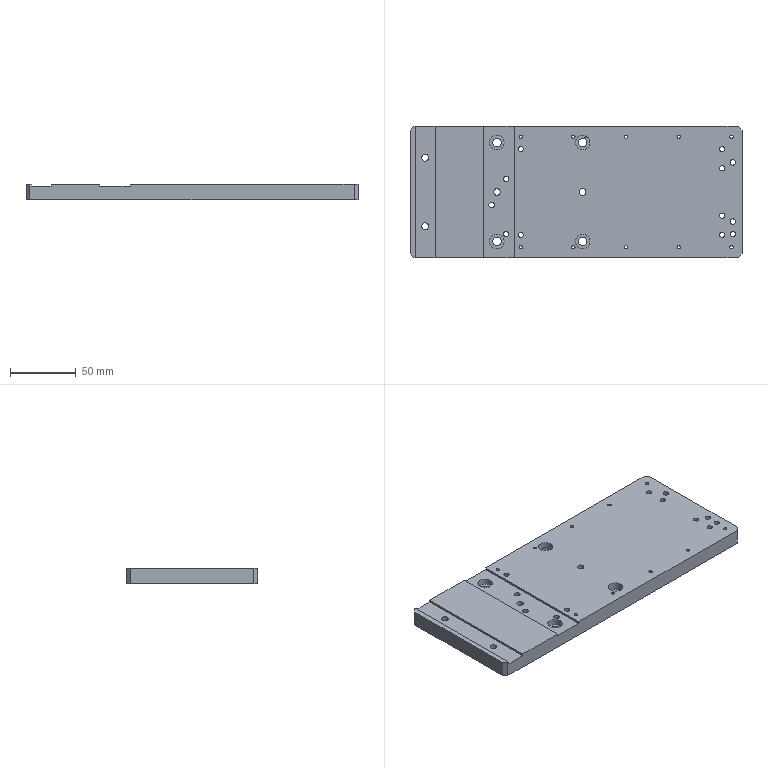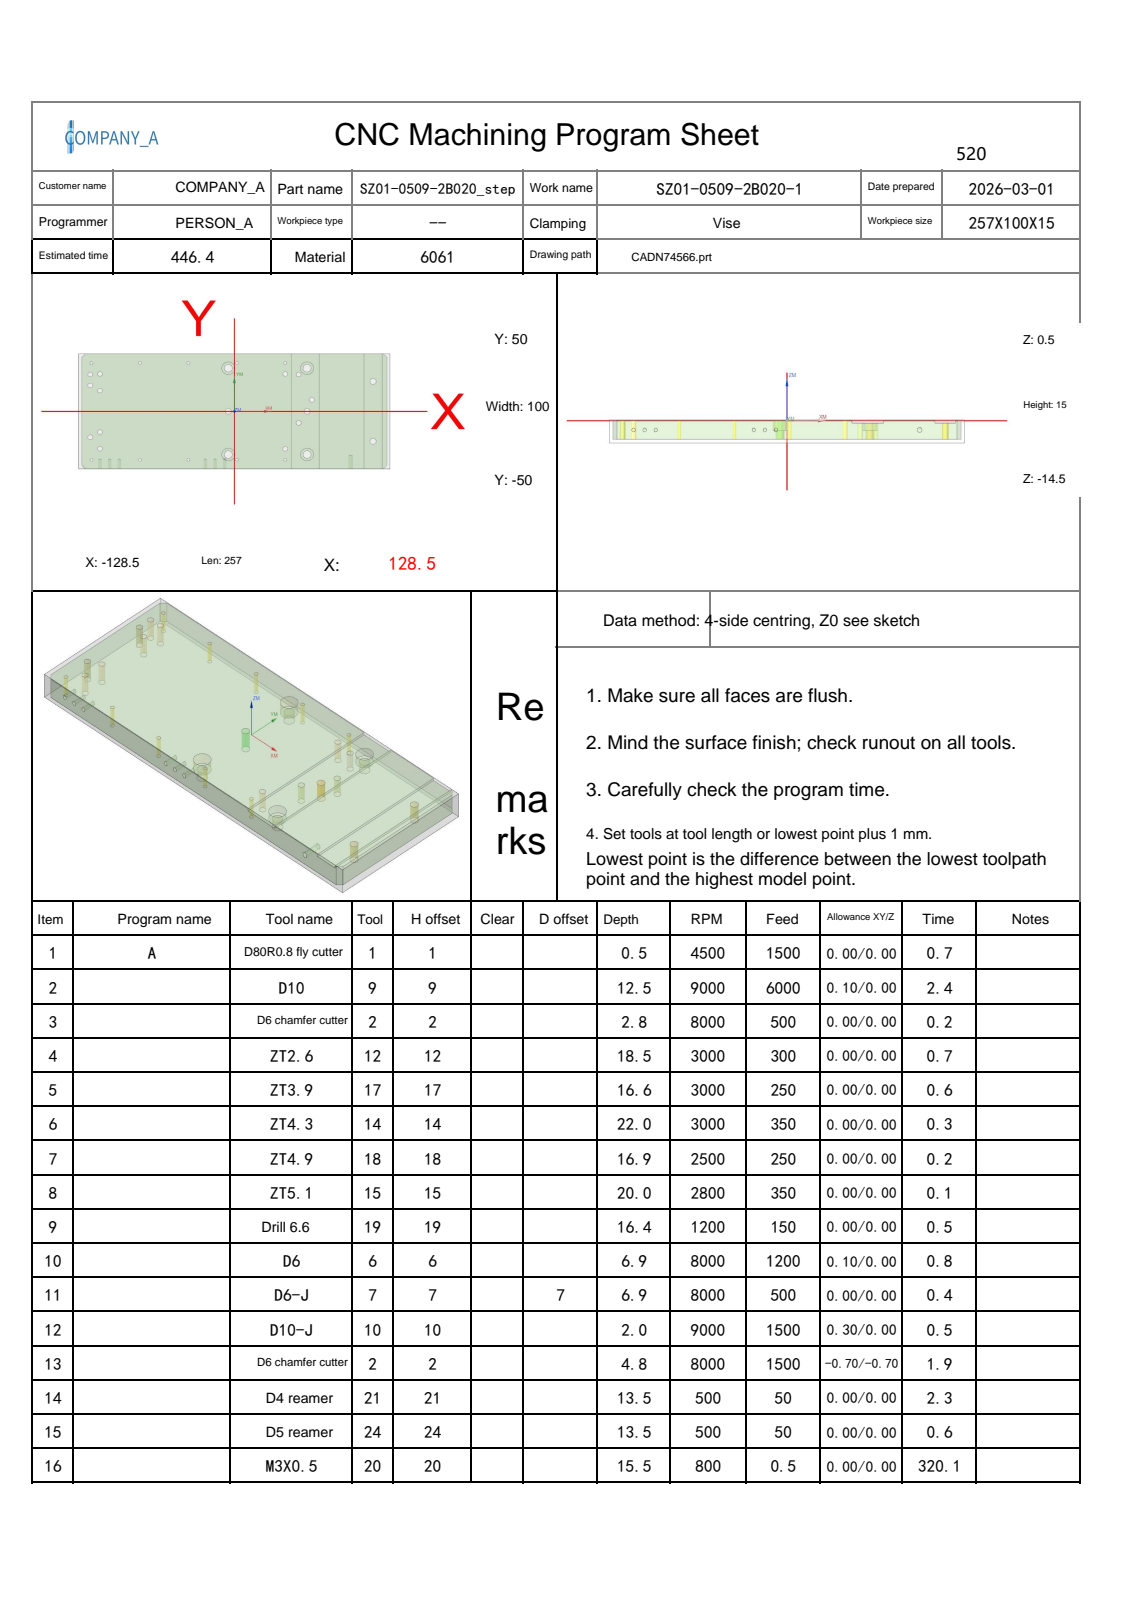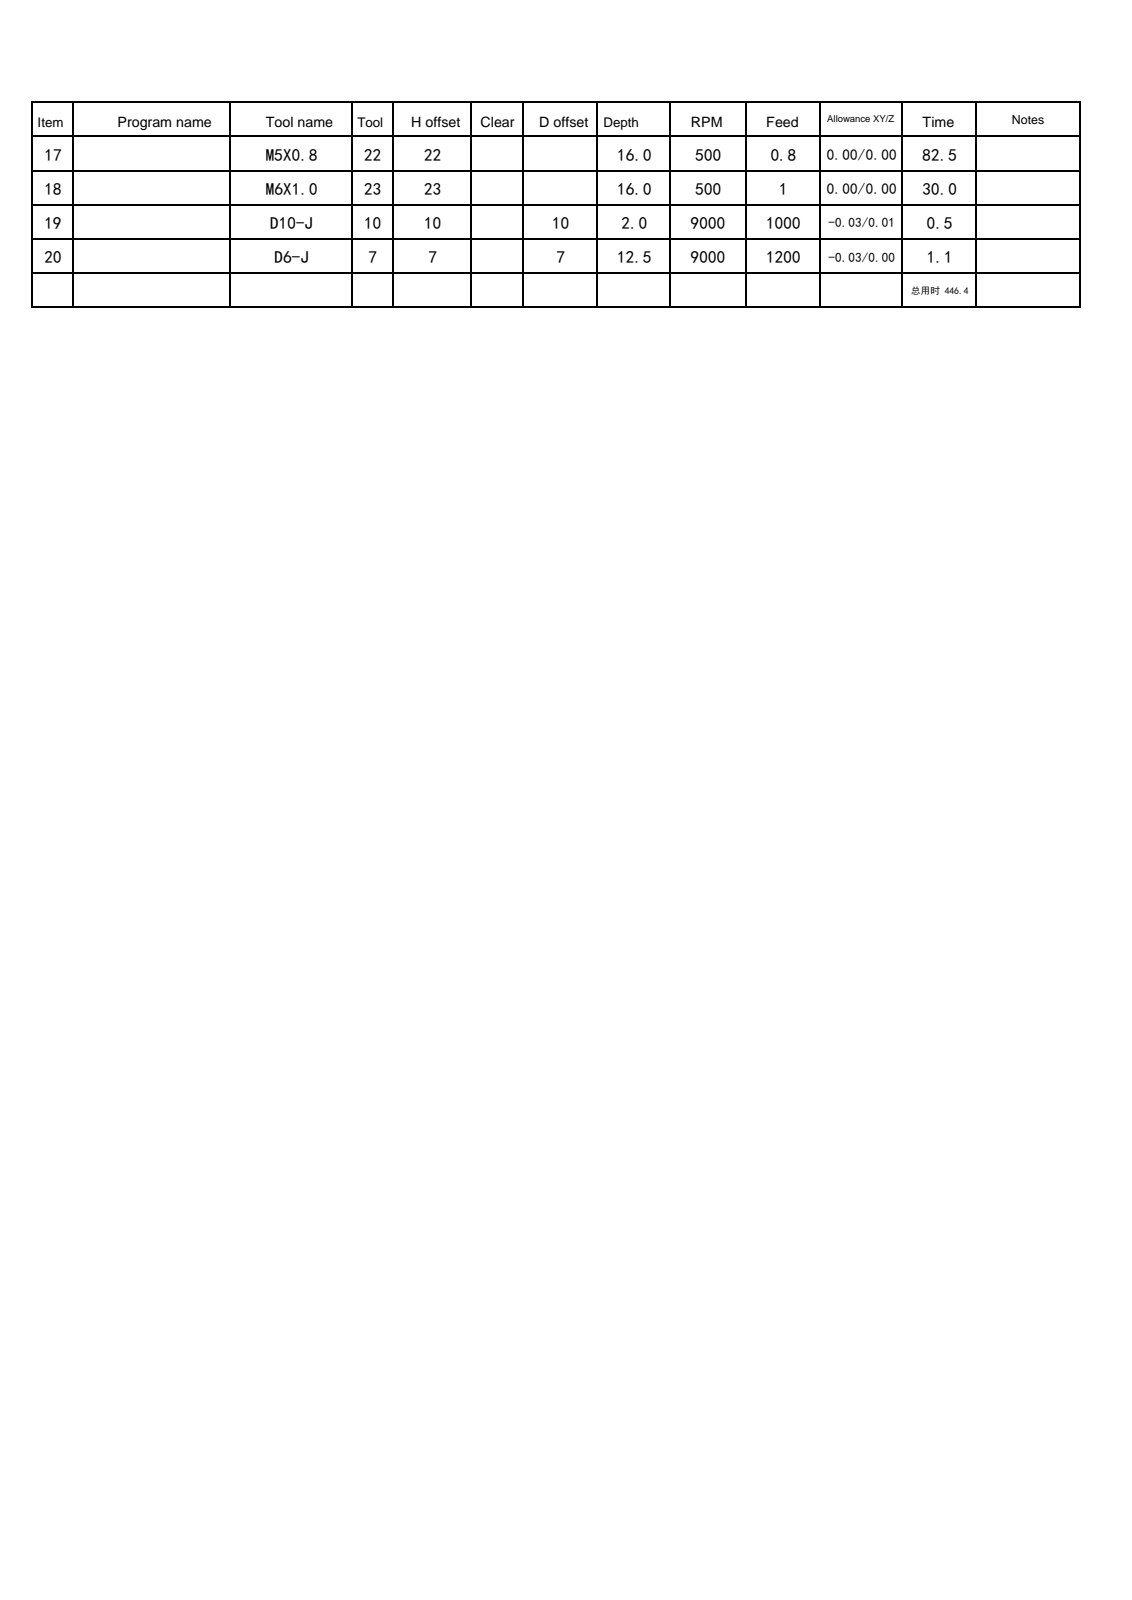NC program | NX | posted by the shop | part box 252 x 100 x 12 mm
Whole program:
%
O0001
(Machine time: 855.61 MIN)
(===Total Tool:17===)
(T1=D80R0.8 fly cutter D=80.  R=0.8  D-  H01 Z=-0.   )
(T9=D10     D=10.  R=0.   D-  H09 Z=-12.  )
(T2=D6 chamfer cutter   D=6.   R=0.   D-  H02 Z=-4.3  )
(T12=ZT2.6  D=2.6  DR_a=118 D-  H12 Z=-18.  )
(T17=ZT3.9  D=3.9  DR_a=120 D-  H17 Z=-16.13)
(T14=ZT4.3  D=4.3  DR_a=118 D-  H14 Z=-21.5 )
(T18=ZT4.9  D=4.9  DR_a=120 D-  H18 Z=-16.41)
(T15=ZT5.1  D=5.1  DR_a=118 D-  H15 Z=-19.53)
(T19=drill 6.6  D=6.6  DR_a=120 D-  H19 Z=-15.91)
(T6=D6      D=6.   R=0.   D-  H06 Z=-6.4  )
(T7=D6-J    D=6.   R=0.   D7  H07 Z=-12.  )
(T10=D10-J  D=10.  R=0.   D-  H10 Z=-1.5  )
(T21=D4 reamer   D=4.   DR_a=180 D-  H21 Z=-13.  )
(T24=D5 reamer   D=5.   DR_a=180 D-  H24 Z=-13.  )
(T20=M3X0.5 D=2.5  DR_a=180 D-  H20 Z=-15.  )
(T22=M5X0.8 D=4.2  DR_a=180 D-  H22 Z=-15.5 )
(T23=M6X1.0 D=5.   DR_a=180 D-  H23 Z=-15.5 )
G80 G90 G17 G49 G40
G91 G28 Z0
M01
N1 T01 M06
(D80R0.8 fly cutter  D=80. R=0.8 H=01 ce=0.00 di=0.00)
G00 G90 G54 X171. Y-45. M03 S4500
G43 H01 Z50.
M08
Z2.
G01 Z0.0 F1500.
X166.
X-166.
Y0.0
X166.
Y45.
X-166.
X-171.
Z2.
G00 Z50.
G91 G28 Z0.0
M05
M09
G91 G28 Z0.0
M01
N2 T09 M06
(D10  D=10. R=0. H=09 ce=0.10 di=0.00)
G00 G90 G54 X0.0 Y-55.1 M03 S8000
G43 H09 Z50.
M08
Z.5
G01 X-123. Z.368 F6000.
G02 X-126.606 Y-53.606 Z.364 I0.0 J5.1
G01 X-129.606 Y-50.606 Z.359
G02 X-131.1 Y-47. Z.355 I3.606 J3.606
G01 Y47. Z.254
G02 X-129.606 Y50.606 Z.25 I5.1 J0.0
G01 X-126.606 Y53.606 Z.245
G02 X-123. Y55.1 Z.241 I3.606 J-3.606
G01 X123. Z-.022
G02 X126.606 Y53.606 Z-.027 I0.0 J-5.1
G01 X129.606 Y50.606 Z-.031
G02 X131.1 Y47. Z-.036 I-3.606 J-3.606
G01 Y-47. Z-.136
G02 X129.606 Y-50.606 Z-.141 I-5.1 J0.0
G01 X126.606 Y-53.606 Z-.145
G02 X123. Y-55.1 Z-.149 I-3.606 J3.606
G01 X-123. Z-.413
G02 X-126.606 Y-53.606 Z-.417 I0.0 J5.1
G01 X-129.606 Y-50.606 Z-.422
G02 X-131.1 Y-47. Z-.426 I3.606 J3.606
G01 Y47. Z-.527
G02 X-129.606 Y50.606 Z-.531 I5.1 J0.0
G01 X-126.606 Y53.606 Z-.536
G02 X-123. Y55.1 Z-.54 I3.606 J-3.606
G01 X123. Z-.804
G02 X126.606 Y53.606 Z-.808 I0.0 J-5.1
G01 X129.606 Y50.606 Z-.813
G02 X131.1 Y47. Z-.817 I-3.606 J-3.606
G01 Y-47. Z-.918
G02 X129.606 Y-50.606 Z-.922 I-5.1 J0.0
G01 X126.606 Y-53.606 Z-.926
G02 X123. Y-55.1 Z-.931 I-3.606 J3.606
G01 X-123. Z-1.194
G02 X-126.606 Y-53.606 Z-1.199 I0.0 J5.1
G01 X-129.606 Y-50.606 Z-1.203
G02 X-131.1 Y-47. Z-1.207 I3.606 J3.606
G01 Y47. Z-1.308
G02 X-129.606 Y50.606 Z-1.312 I5.1 J0.0
G01 X-126.606 Y53.606 Z-1.317
G02 X-123. Y55.1 Z-1.321 I3.606 J-3.606
G01 X123. Z-1.585
G02 X126.606 Y53.606 Z-1.589 I0.0 J-5.1
G01 X129.606 Y50.606 Z-1.594
G02 X131.1 Y47. Z-1.598 I-3.606 J-3.606
G01 Y-47. Z-1.699
G02 X129.606 Y-50.606 Z-1.703 I-5.1 J0.0
G01 X126.606 Y-53.606 Z-1.708
G02 X123. Y-55.1 Z-1.712 I-3.606 J3.606
G01 X-123. Z-1.976
G02 X-126.606 Y-53.606 Z-1.98 I0.0 J5.1
G01 X-129.606 Y-50.606 Z-1.984
G02 X-131.1 Y-47. Z-1.989 I3.606 J3.606
G01 Y47. Z-2.089
G02 X-129.606 Y50.606 Z-2.094 I5.1 J0.0
G01 X-126.606 Y53.606 Z-2.098
G02 X-123. Y55.1 Z-2.103 I3.606 J-3.606
G01 X123. Z-2.366
G02 X126.606 Y53.606 Z-2.37 I0.0 J-5.1
G01 X129.606 Y50.606 Z-2.375
G02 X131.1 Y47. Z-2.379 I-3.606 J-3.606
G01 Y-47. Z-2.48
G02 X129.606 Y-50.606 Z-2.484 I-5.1 J0.0
G01 X126.606 Y-53.606 Z-2.489
G02 X123. Y-55.1 Z-2.493 I-3.606 J3.606
G01 X-123. Z-2.757
G02 X-126.606 Y-53.606 Z-2.761 I0.0 J5.1
G01 X-129.606 Y-50.606 Z-2.766
G02 X-131.1 Y-47. Z-2.77 I3.606 J3.606
G01 Y47. Z-2.871
G02 X-129.606 Y50.606 Z-2.875 I5.1 J0.0
G01 X-126.606 Y53.606 Z-2.88
G02 X-123. Y55.1 Z-2.884 I3.606 J-3.606
G01 X123. Z-3.147
G02 X126.606 Y53.606 Z-3.152 I0.0 J-5.1
G01 X129.606 Y50.606 Z-3.156
G02 X131.1 Y47. Z-3.161 I-3.606 J-3.606
G01 Y-47. Z-3.261
G02 X129.606 Y-50.606 Z-3.266 I-5.1 J0.0
G01 X126.606 Y-53.606 Z-3.27
G02 X123. Y-55.1 Z-3.274 I-3.606 J3.606
G01 X-123. Z-3.538
G02 X-126.606 Y-53.606 Z-3.542 I0.0 J5.1
G01 X-129.606 Y-50.606 Z-3.547
G02 X-131.1 Y-47. Z-3.551 I3.606 J3.606
G01 Y47. Z-3.652
G02 X-129.606 Y50.606 Z-3.656 I5.1 J0.0
G01 X-126.606 Y53.606 Z-3.661
G02 X-123. Y55.1 Z-3.665 I3.606 J-3.606
G01 X123. Z-3.929
G02 X126.606 Y53.606 Z-3.933 I0.0 J-5.1
G01 X129.606 Y50.606 Z-3.938
G02 X131.1 Y47. Z-3.942 I-3.606 J-3.606
G01 Y-47. Z-4.043
G02 X129.606 Y-50.606 Z-4.047 I-5.1 J0.0
G01 X126.606 Y-53.606 Z-4.051
G02 X123. Y-55.1 Z-4.056 I-3.606 J3.606
G01 X-123. Z-4.319
G02 X-126.606 Y-53.606 Z-4.324 I0.0 J5.1
G01 X-129.606 Y-50.606 Z-4.328
G02 X-131.1 Y-47. Z-4.332 I3.606 J3.606
G01 Y47. Z-4.433
G02 X-129.606 Y50.606 Z-4.437 I5.1 J0.0
G01 X-126.606 Y53.606 Z-4.442
G02 X-123. Y55.1 Z-4.446 I3.606 J-3.606
G01 X123. Z-4.71
G02 X126.606 Y53.606 Z-4.714 I0.0 J-5.1
G01 X129.606 Y50.606 Z-4.719
G02 X131.1 Y47. Z-4.723 I-3.606 J-3.606
G01 Y-47. Z-4.824
G02 X129.606 Y-50.606 Z-4.828 I-5.1 J0.0
G01 X126.606 Y-53.606 Z-4.833
G02 X123. Y-55.1 Z-4.837 I-3.606 J3.606
G01 X-123. Z-5.101
G02 X-126.606 Y-53.606 Z-5.105 I0.0 J5.1
G01 X-129.606 Y-50.606 Z-5.109
G02 X-131.1 Y-47. Z-5.114 I3.606 J3.606
G01 Y47. Z-5.214
G02 X-129.606 Y50.606 Z-5.219 I5.1 J0.0
G01 X-126.606 Y53.606 Z-5.223
G02 X-123. Y55.1 Z-5.228 I3.606 J-3.606
G01 X123. Z-5.491
G02 X126.606 Y53.606 Z-5.495 I0.0 J-5.1
G01 X129.606 Y50.606 Z-5.5
G02 X131.1 Y47. Z-5.504 I-3.606 J-3.606
G01 Y-47. Z-5.605
G02 X129.606 Y-50.606 Z-5.609 I-5.1 J0.0
G01 X126.606 Y-53.606 Z-5.614
G02 X123. Y-55.1 Z-5.618 I-3.606 J3.606
G01 X-123. Z-5.882
G02 X-126.606 Y-53.606 Z-5.886 I0.0 J5.1
G01 X-129.606 Y-50.606 Z-5.891
G02 X-131.1 Y-47. Z-5.895 I3.606 J3.606
G01 Y47. Z-5.996
G02 X-129.606 Y50.606 Z-6. I5.1 J0.0
G01 X-126.606 Y53.606 Z-6.005
G02 X-123. Y55.1 Z-6.009 I3.606 J-3.606
G01 X123. Z-6.272
G02 X126.606 Y53.606 Z-6.277 I0.0 J-5.1
G01 X129.606 Y50.606 Z-6.281
G02 X131.1 Y47. Z-6.286 I-3.606 J-3.606
G01 Y-47. Z-6.386
G02 X129.606 Y-50.606 Z-6.391 I-5.1 J0.0
G01 X126.606 Y-53.606 Z-6.395
G02 X123. Y-55.1 Z-6.399 I-3.606 J3.606
G01 X-123. Z-6.663
G02 X-126.606 Y-53.606 Z-6.667 I0.0 J5.1
G01 X-129.606 Y-50.606 Z-6.672
G02 X-131.1 Y-47. Z-6.676 I3.606 J3.606
G01 Y47. Z-6.777
G02 X-129.606 Y50.606 Z-6.781 I5.1 J0.0
G01 X-126.606 Y53.606 Z-6.786
G02 X-123. Y55.1 Z-6.79 I3.606 J-3.606
G01 X123. Z-7.054
G02 X126.606 Y53.606 Z-7.058 I0.0 J-5.1
G01 X129.606 Y50.606 Z-7.063
G02 X131.1 Y47. Z-7.067 I-3.606 J-3.606
G01 Y-47. Z-7.168
G02 X129.606 Y-50.606 Z-7.172 I-5.1 J0.0
G01 X126.606 Y-53.606 Z-7.176
G02 X123. Y-55.1 Z-7.181 I-3.606 J3.606
G01 X-123. Z-7.444
G02 X-126.606 Y-53.606 Z-7.449 I0.0 J5.1
G01 X-129.606 Y-50.606 Z-7.453
G02 X-131.1 Y-47. Z-7.457 I3.606 J3.606
G01 Y47. Z-7.558
G02 X-129.606 Y50.606 Z-7.562 I5.1 J0.0
G01 X-126.606 Y53.606 Z-7.567
G02 X-123. Y55.1 Z-7.571 I3.606 J-3.606
G01 X123. Z-7.835
G02 X126.606 Y53.606 Z-7.839 I0.0 J-5.1
G01 X129.606 Y50.606 Z-7.844
G02 X131.1 Y47. Z-7.848 I-3.606 J-3.606
G01 Y-47. Z-7.949
G02 X129.606 Y-50.606 Z-7.953 I-5.1 J0.0
G01 X126.606 Y-53.606 Z-7.958
G02 X123. Y-55.1 Z-7.962 I-3.606 J3.606
G01 X-123. Z-8.226
G02 X-126.606 Y-53.606 Z-8.23 I0.0 J5.1
G01 X-129.606 Y-50.606 Z-8.234
G02 X-131.1 Y-47. Z-8.239 I3.606 J3.606
G01 Y47. Z-8.339
G02 X-129.606 Y50.606 Z-8.344 I5.1 J0.0
G01 X-126.606 Y53.606 Z-8.348
G02 X-123. Y55.1 Z-8.353 I3.606 J-3.606
G01 X123. Z-8.616
G02 X126.606 Y53.606 Z-8.62 I0.0 J-5.1
G01 X129.606 Y50.606 Z-8.625
G02 X131.1 Y47. Z-8.629 I-3.606 J-3.606
G01 Y-47. Z-8.73
G02 X129.606 Y-50.606 Z-8.734 I-5.1 J0.0
G01 X126.606 Y-53.606 Z-8.739
G02 X123. Y-55.1 Z-8.743 I-3.606 J3.606
G01 X-123. Z-9.007
G02 X-126.606 Y-53.606 Z-9.011 I0.0 J5.1
G01 X-129.606 Y-50.606 Z-9.016
G02 X-131.1 Y-47. Z-9.02 I3.606 J3.606
G01 Y47. Z-9.121
G02 X-129.606 Y50.606 Z-9.125 I5.1 J0.0
G01 X-126.606 Y53.606 Z-9.13
G02 X-123. Y55.1 Z-9.134 I3.606 J-3.606
G01 X123. Z-9.397
G02 X126.606 Y53.606 Z-9.402 I0.0 J-5.1
G01 X129.606 Y50.606 Z-9.406
G02 X131.1 Y47. Z-9.411 I-3.606 J-3.606
G01 Y-47. Z-9.511
G02 X129.606 Y-50.606 Z-9.516 I-5.1 J0.0
G01 X126.606 Y-53.606 Z-9.52
G02 X123. Y-55.1 Z-9.524 I-3.606 J3.606
G01 X-123. Z-9.788
G02 X-126.606 Y-53.606 Z-9.792 I0.0 J5.1
G01 X-129.606 Y-50.606 Z-9.797
G02 X-131.1 Y-47. Z-9.801 I3.606 J3.606
G01 Y47. Z-9.902
G02 X-129.606 Y50.606 Z-9.906 I5.1 J0.0
G01 X-126.606 Y53.606 Z-9.911
G02 X-123. Y55.1 Z-9.915 I3.606 J-3.606
G01 X123. Z-10.179
G02 X126.606 Y53.606 Z-10.183 I0.0 J-5.1
G01 X129.606 Y50.606 Z-10.188
G02 X131.1 Y47. Z-10.192 I-3.606 J-3.606
G01 Y-47. Z-10.293
G02 X129.606 Y-50.606 Z-10.297 I-5.1 J0.0
G01 X126.606 Y-53.606 Z-10.301
G02 X123. Y-55.1 Z-10.306 I-3.606 J3.606
G01 X-123. Z-10.569
G02 X-126.606 Y-53.606 Z-10.574 I0.0 J5.1
G01 X-129.606 Y-50.606 Z-10.578
G02 X-131.1 Y-47. Z-10.582 I3.606 J3.606
G01 Y47. Z-10.683
G02 X-129.606 Y50.606 Z-10.687 I5.1 J0.0
G01 X-126.606 Y53.606 Z-10.692
G02 X-123. Y55.1 Z-10.696 I3.606 J-3.606
G01 X123. Z-10.96
G02 X126.606 Y53.606 Z-10.964 I0.0 J-5.1
G01 X129.606 Y50.606 Z-10.969
G02 X131.1 Y47. Z-10.973 I-3.606 J-3.606
G01 Y-47. Z-11.074
G02 X129.606 Y-50.606 Z-11.078 I-5.1 J0.0
G01 X126.606 Y-53.606 Z-11.083
G02 X123. Y-55.1 Z-11.087 I-3.606 J3.606
G01 X-123. Z-11.351
G02 X-126.606 Y-53.606 Z-11.355 I0.0 J5.1
G01 X-129.606 Y-50.606 Z-11.359
G02 X-131.1 Y-47. Z-11.364 I3.606 J3.606
G01 Y47. Z-11.464
G02 X-129.606 Y50.606 Z-11.469 I5.1 J0.0
G01 X-126.606 Y53.606 Z-11.473
G02 X-123. Y55.1 Z-11.478 I3.606 J-3.606
G01 X123. Z-11.741
G02 X126.606 Y53.606 Z-11.745 I0.0 J-5.1
G01 X129.606 Y50.606 Z-11.75
G02 X131.1 Y47. Z-11.754 I-3.606 J-3.606
G01 Y-47. Z-11.855
G02 X129.606 Y-50.606 Z-11.859 I-5.1 J0.0
G01 X126.606 Y-53.606 Z-11.864
G02 X123. Y-55.1 Z-11.868 I-3.606 J3.606
G01 X0.0 Z-12.
X-123.
G02 X-126.606 Y-53.606 I0.0 J5.1
G01 X-129.606 Y-50.606
G02 X-131.1 Y-47. I3.606 J3.606
G01 Y47.
G02 X-129.606 Y50.606 I5.1 J0.0
G01 X-126.606 Y53.606
G02 X-123. Y55.1 I3.606 J-3.606
G01 X123.
G02 X126.606 Y53.606 I0.0 J-5.1
G01 X129.606 Y50.606
G02 X131.1 Y47. I-3.606 J-3.606
G01 Y-47.
G02 X129.606 Y-50.606 I-5.1 J0.0
G01 X126.606 Y-53.606
G02 X123. Y-55.1 I-3.606 J3.606
G01 X0.0
X-.5
Z-11.
G00 Z50.
G00 G90 X58.5 Y58. M03 S9000
Z50.
Z.033
G01 Z-.467 F6000.
Y46.5
X56.6
Y-46.5
X60.4
Y46.5
X58.5
Y51.
X52.1
Y-51.
X64.9
Y51.
X58.5
X58.
Z.033
G00 Z.5
X58.5 Y58.
Z-.433
G01 Z-.933
Y46.5
X56.6
Y-46.5
X60.4
Y46.5
X58.5
Y51.
X52.1
Y-51.
X64.9
Y51.
X58.5
X58.
Z-.433
G00 Z.033
X58.5 Y58.
Z-.9
G01 Z-1.4
Y46.5
X56.6
Y-46.5
X60.4
Y46.5
X58.5
Y51.
X52.1
Y-51.
X64.9
Y51.
X58.5
X58.
Z-.9
G00 Z50.
G00 G90 X114.5 Y-58.1 M03 S9000
Z50.
Z.033
G01 Z-.467 F6000.
Y-51.
X116.9
Y51.
X112.1
Y-51.
X114.5
X115.
Z.033
G00 Z.5
X114.5 Y-58.1
Z-.433
G01 Z-.933
Y-51.
X116.9
Y51.
X112.1
Y-51.
X114.5
X115.
Z-.433
G00 Z.033
X114.5 Y-58.1
Z-.9
G01 Z-1.4
Y-51.
X116.9
Y51.
X112.1
Y-51.
X114.5
X115.
Z-.9
G00 Z50.
G91 G28 Z0.0
M05
M09
G91 G28 Z0.0
M01
N3 T02 M06
(D6 chamfer cutter  D=6. R=0. H=02 ce=0.00 di=0.10)
G00 G90 G54 X114.5 Y26. M03 S8000
G43 H02 Z50.
M08
G98 G81 X114.5 Y26. Z-2.3 R-.5 F500.
Y-26.
X60. Y-37.5
X42. Y-42. Z-.8 R1.
Y-32.5
X53. Y-10. Z-2.3 R-.5
X60. Y0.0
X64. Y10.
X60. Y37.5
X53. Y32.
X42. Y32.5 Z-.8 R1.
Y42.
X2.
X-5. Y37.5
X-38. Y42.
X-78.
X-111. Y32.5
X-118. Y42.
X-119. Y32.
Y22.5
X-111. Y18.
Y-18.
X-119. Y-22.5
X-111. Y-32.5
X-118. Y-42.
X-78.
X-38.
X-5. Y-37.5
X2. Y-42.
X-5. Y0.0
G80
G00 Z50.
G91 G28 Z0.0
M05
M09
G91 G28 Z0.0
M01
N4 T12 M06
(ZT2.6 D=2.6 DR_a=118 H=12)
G00 G90 G54 X-118. Y-42. M03 S3000
G43 H12 Z50.
M08
G98 G83 X-118. Y-42. Z-18. R1. F300. Q2.
X-78.
X-38.
X2.
X42.
Y42.
X2.
X-38.
X-78.
X-118.
G80
G00 Z50.
G91 G28 Z0.0
M05
M09
G91 G28 Z0.0
M01
N5 T17 M06
(ZT3.9 D=3.9 DR_a=120 H=17)
G00 G90 G54 X-119. Y32. M03 S3000
G43 H17 Z50.
M08
G98 G83 X-119. Y32. Z-16.126 R1. F250. Q2.
X-111. Y32.5
Y18.
Y-18.
Y-32.5
X42.
Y32.5
G98 G83 X53. Y32. Z-16.126 R-.5 Q2.
G80
G00 Z50.
G91 G28 Z0.0
M05
M09
G91 G28 Z0.0
M01
N6 T14 M06
(ZT4.3 D=4.3 DR_a=118 H=14)
G00 G90 G54 X-119. Y22.5 M03 S3000
G43 H14 Z50.
M08
G98 G83 X-119. Y22.5 Z-20. R1. F350. Q3.
Y-22.5
X53. Y-10. Z-21.5 R-.5
X64. Y10.
G80
G00 Z50.
G91 G28 Z0.0
M05
M09
G91 G28 Z0.0
M01
N7 T18 M06
(ZT4.9 D=4.9 DR_a=120 H=18)
G00 G90 G54 X-5. Y0.0 M03 S2500
G43 H18 Z50.
M08
G98 G83 X-5. Y0.0 Z-16.415 R1. F250. Q2.
G98 G83 X60. Y0.0 Z-16.415 R-.5 Q2.
G80
G00 Z50.
G91 G28 Z0.0
M05
M09
G91 G28 Z0.0
M01
N8 T15 M06
(ZT5.1 D=5.1 DR_a=118 H=15)
G00 G90 G54 X114.5 Y26. M03 S2800
G43 H15 Z50.
M08
G98 G83 X114.5 Y26. Z-19.532 R-.5 F350. Q3.
Y-26.
G80
G00 Z50.
G91 G28 Z0.0
M05
M09
G91 G28 Z0.0
M01
N9 T19 M06
(Drill 6.6 D=6.6 DR_a=120 H=19)
G00 G90 G54 X-5. Y37.5 M03 S1200
G43 H19 Z50.
M08
G98 G83 X-5. Y37.5 Z-15.905 R1. F150. Q2.
G98 G83 X60. Y37.5 Z-15.905 R-.5 Q2.
Y-37.5
G98 G83 X-5. Y-37.5 Z-15.905 R1. Q2.
G80
G00 Z50.
G91 G28 Z0.0
M05
M09
G91 G28 Z0.0
M01
N10 T06 M06
(D6  D=6. R=0. H=06 ce=0.10 di=0.00)
G00 G90 G54 X-5. Y37.5 M03 S8000
G43 H06 Z50.
M08
Z.5
G03 X-6.2 Y38.7 I-1.2 J0.0 F1200.
X-7.4 Y37.5 I0.0 J-1.2
X-7.4 Y37.5 Z0.0 I2.4 J0.0
X-7.4 Y37.5 Z-.5 I2.4 J0.0
X-7.4 Y37.5 Z-1. I2.4 J0.0
X-7.4 Y37.5 Z-1.5 I2.4 J0.0
X-7.4 Y37.5 Z-2. I2.4 J0.0
X-7.4 Y37.5 Z-2.5 I2.4 J0.0
X-7.4 Y37.5 Z-3. I2.4 J0.0
X-7.4 Y37.5 Z-3.5 I2.4 J0.0
X-7.4 Y37.5 Z-4. I2.4 J0.0
X-7.4 Y37.5 Z-4.5 I2.4 J0.0
X-7.4 Y37.5 Z-5. I2.4 J0.0
X-7.4 Y37.5 Z-5.5 I2.4 J0.0
X-7.4 Y37.5 Z-6. I2.4 J0.0
X-5.742 Y39.783 Z-6.4 I2.4 J0.0
X-7.4 Y37.5 I.742 J-2.283
X-5. Y35.1 I2.4 J0.0
X-2.6 Y37.5 I0.0 J2.4
X-5. Y39.9 I-2.4 J0.0
X-5.742 Y39.783 I0.0 J-2.4
X-6.571 Y38.641 I.371 J-1.141
X-5.371 Y37.441 I1.2 J0.0
X-5. Y37.5 I0.0 J1.2
G00 Z50.
Y-37.5
Z.5
G03 X-6.2 Y-36.3 I-1.2 J0.0
X-7.4 Y-37.5 I0.0 J-1.2
X-7.4 Y-37.5 Z0.0 I2.4 J0.0
X-7.4 Y-37.5 Z-.5 I2.4 J0.0
X-7.4 Y-37.5 Z-1. I2.4 J0.0
X-7.4 Y-37.5 Z-1.5 I2.4 J0.0
X-7.4 Y-37.5 Z-2. I2.4 J0.0
X-7.4 Y-37.5 Z-2.5 I2.4 J0.0
X-7.4 Y-37.5 Z-3. I2.4 J0.0
X-7.4 Y-37.5 Z-3.5 I2.4 J0.0
X-7.4 Y-37.5 Z-4. I2.4 J0.0
X-7.4 Y-37.5 Z-4.5 I2.4 J0.0
X-7.4 Y-37.5 Z-5. I2.4 J0.0
X-7.4 Y-37.5 Z-5.5 I2.4 J0.0
X-7.4 Y-37.5 Z-6. I2.4 J0.0
X-5.742 Y-35.217 Z-6.4 I2.4 J0.0
X-7.4 Y-37.5 I.742 J-2.283
X-5. Y-39.9 I2.4 J0.0
X-2.6 Y-37.5 I0.0 J2.4
X-5. Y-35.1 I-2.4 J0.0
X-5.742 Y-35.217 I0.0 J-2.4
X-6.571 Y-36.359 I.371 J-1.141
X-5.371 Y-37.559 I1.2 J0.0
X-5. Y-37.5 I0.0 J1.2
G00 Z50.
G00 G90 X60. Y37.5 M03 S8000
Z50.
Z-1.
G03 X58.8 Y38.7 I-1.2 J0.0 F1200.
X57.6 Y37.5 I0.0 J-1.2
X57.6 Y37.5 Z-1.5 I2.4 J0.0
X57.6 Y37.5 Z-2. I2.4 J0.0
X57.6 Y37.5 Z-2.5 I2.4 J0.0
X57.6 Y37.5 Z-3. I2.4 J0.0
X57.6 Y37.5 Z-3.5 I2.4 J0.0
X57.6 Y37.5 Z-4. I2.4 J0.0
X57.6 Y37.5 Z-4.5 I2.4 J0.0
X57.6 Y37.5 Z-5. I2.4 J0.0
X57.6 Y37.5 Z-5.5 I2.4 J0.0
X57.6 Y37.5 Z-6. I2.4 J0.0
X59.258 Y39.783 Z-6.4 I2.4 J0.0
X57.6 Y37.5 I.742 J-2.283
X60. Y35.1 I2.4 J0.0
X62.4 Y37.5 I0.0 J2.4
X60. Y39.9 I-2.4 J0.0
X59.258 Y39.783 I0.0 J-2.4
X58.429 Y38.641 I.371 J-1.141
X59.629 Y37.441 I1.2 J0.0
X60. Y37.5 I0.0 J1.2
G00 Z50.
Y-37.5
Z-1.
G03 X58.8 Y-36.3 I-1.2 J0.0
X57.6 Y-37.5 I0.0 J-1.2
X57.6 Y-37.5 Z-1.5 I2.4 J0.0
X57.6 Y-37.5 Z-2. I2.4 J0.0
X57.6 Y-37.5 Z-2.5 I2.4 J0.0
X57.6 Y-37.5 Z-3. I2.4 J0.0
X57.6 Y-37.5 Z-3.5 I2.4 J0.0
X57.6 Y-37.5 Z-4. I2.4 J0.0
X57.6 Y-37.5 Z-4.5 I2.4 J0.0
X57.6 Y-37.5 Z-5. I2.4 J0.0
X57.6 Y-37.5 Z-5.5 I2.4 J0.0
X57.6 Y-37.5 Z-6. I2.4 J0.0
X59.258 Y-35.217 Z-6.4 I2.4 J0.0
X57.6 Y-37.5 I.742 J-2.283
X60. Y-39.9 I2.4 J0.0
X62.4 Y-37.5 I0.0 J2.4
X60. Y-35.1 I-2.4 J0.0
X59.258 Y-35.217 I0.0 J-2.4
X58.429 Y-36.359 I.371 J-1.141
X59.629 Y-37.559 I1.2 J0.0
X60. Y-37.5 I0.0 J1.2
G00 Z50.
G91 G28 Z0.0
M05
M09
G91 G28 Z0.0
M01
N11 T07 M06
(D6-J  D=6. R=0. H=07 ce=0.00 di=0.00)
G00 G90 G54 X-5. Y37.5 M03 S8000
G43 H07 Z50.
M08
Z0.0
G41 D07
G01 X-5.032 Y37.697 F500.
G03 X-6.258 Y38.742 I-1.226 J-.197
X-7.5 Y37.5 I0.0 J-1.242
X-7.5 Y37.5 Z-5. I2.5 J0.0
X-4.532 Y35.044 Z-6.4 I2.5 J0.0
X-2.5 Y37.5 I-.468 J2.456
X-5. Y40. I-2.5 J0.0
X-7.5 Y37.5 I0.0 J-2.5
X-5. Y35. I2.5 J0.0
X-4.532 Y35.044 I0.0 J2.5
X-3.522 Y36.264 I-.233 J1.22
X-4.764 Y37.506 I-1.242 J0.0
G01 X-4.8
G40 X-5. Y37.5
G00 Z50.
Y-37.5
Z0.0
G41 D07
G01 X-5.032 Y-37.303
G03 X-6.258 Y-36.258 I-1.226 J-.197
X-7.5 Y-37.5 I0.0 J-1.242
X-7.5 Y-37.5 Z-5. I2.5 J0.0
X-4.532 Y-39.956 Z-6.4 I2.5 J0.0
X-2.5 Y-37.5 I-.468 J2.456
X-5. Y-35. I-2.5 J0.0
X-7.5 Y-37.5 I0.0 J-2.5
X-5. Y-40. I2.5 J0.0
X-4.532 Y-39.956 I0.0 J2.5
X-3.522 Y-38.736 I-.233 J1.22
X-4.764 Y-37.494 I-1.242 J0.0
G01 X-4.8
G40 X-5. Y-37.5
G00 Z50.
G00 G90 X60. Y37.5 M03 S8000
Z50.
Z-1.5
G41 D07
G01 X59.968 Y37.697 F500.
G03 X58.742 Y38.742 I-1.226 J-.197
X57.5 Y37.5 I0.0 J-1.242
X57.52 Y37.813 Z-6.4 I2.5 J0.0
X57.5 Y37.5 I2.48 J-.313
X60. Y35. I2.5 J0.0
X62.5 Y37.5 I0.0 J2.5
X60. Y40. I-2.5 J0.0
X57.52 Y37.813 I0.0 J-2.5
G01 X57.51 Y37.658
G03 X58.752 Y36.416 I1.242 J0.0
X59.944 Y37.308 I0.0 J1.242
G01 G40 X60. Y37.5
G00 Z50.
Y-37.5
Z-1.5
G41 D07
G01 X59.968 Y-37.303
G03 X58.742 Y-36.258 I-1.226 J-.197
X57.5 Y-37.5 I0.0 J-1.242
X57.52 Y-37.187 Z-6.4 I2.5 J0.0
X57.5 Y-37.5 I2.48 J-.313
X60. Y-40. I2.5 J0.0
X62.5 Y-37.5 I0.0 J2.5
X60. Y-35. I-2.5 J0.0
X57.52 Y-37.187 I0.0 J-2.5
G01 X57.51 Y-37.342
G03 X58.752 Y-38.584 I1.242 J0.0
X59.944 Y-37.692 I0.0 J1.242
G01 G40 X60. Y-37.5
G00 Z50.
G91 G28 Z0.0
M05
M09
G91 G28 Z0.0
M01
N12 T10 M06
(D10-J  D=10. R=0. H=10 ce=0.30 di=0.00)
G00 G90 G54 X58.5 Y58. M03 S9000
G43 H10 Z50.
M08
Z-1.
G01 Z-1.5 F1500.
Y51.
X64.7
Y-51.
X52.3
Y51.
X58.5
Y46.5
X60.2
Y-46.5
X56.8
Y46.5
X58.5
X59.
Y58.
Z-1.
G00 Z50.
G00 G90 X114.5 Y58.3 M03 S9000
Z50.
Z-1.
G01 Z-1.5 F1500.
Y51.
X116.7
Y-51.
X112.3
Y51.
X114.5
X115.
Y58.3
Z-1.
G00 Z50.
G91 G28 Z0.0
M05
M09
G91 G28 Z0.0
M01
N13 T02 M06
(D6 chamfer cutter  D=6. R=0. H=02 ce=0.00 di=0.00)
G00 G90 G54 X-118. Y-42. M03 S8000
G43 H02 Z50.
M08
G98 G81 X-118. Y-42. Z-1.75 R3. F500.
X-78.
X-38.
X2.
X42.
Y42.
X2.
X-38.
X-78.
X-118.
G80
G00 Z50.
G00 G90 X-119. Y32. M03 S8000
Z50.
G98 G81 X-119. Y32. Z-2.3 R3. F500.
X-111. Y32.5
Y18.
Y-18.
Y-32.5
X42.
Y32.5
X53. Y32. Z-3.8 R1.5
G80
G00 Z50.
G00 G90 X-118.907 Y21.806 M03 S8000
Z50.
Z-.5
G01 Z-1. F500.
X-118.8 Y21.
G03 X-117.3 Y22.5 I0.0 J1.5
X-119. Y24.2 I-1.7 J0.0
X-120.7 Y22.5 I0.0 J-1.7
X-119. Y20.8 I1.7 J0.0
X-117.3 Y22.5 I0.0 J1.7
X-118.8 Y24. I-1.5 J0.0
G01 X-118.907 Y23.194
Z-.5
G00 Z50.
Y-23.194
Z-.5
G01 Z-1.
X-118.8 Y-24.
G03 X-117.3 Y-22.5 I0.0 J1.5
X-119. Y-20.8 I-1.7 J0.0
X-120.7 Y-22.5 I0.0 J-1.7
X-119. Y-24.2 I1.7 J0.0
X-117.3 Y-22.5 I0.0 J1.7
X-118.8 Y-21. I-1.5 J0.0
G01 X-118.907 Y-21.806
Z-.5
G00 Z50.
G00 G90 X-4.843 Y-.784 M03 S8000
Z50.
Z-.5
G01 Z-1. F500.
X-4.7 Y-1.5
G03 X-3.2 Y0.0 I0.0 J1.5
X-5. Y1.8 I-1.8 J0.0
X-6.8 Y0.0 I0.0 J-1.8
X-5. Y-1.8 I1.8 J0.0
X-3.2 Y0.0 I0.0 J1.8
X-4.7 Y1.5 I-1.5 J0.0
G01 X-4.843 Y.784
Z-.5
G00 Z50.
G00 G90 X114.957 Y24.945 M03 S8000
Z50.
Z-2.1
G01 Z-2.6 F500.
X115.15 Y24.5
G03 X116.65 Y26. I0.0 J1.5
X114.5 Y28.15 I-2.15 J0.0
X112.35 Y26. I0.0 J-2.15
X114.5 Y23.85 I2.15 J0.0
X116.65 Y26. I0.0 J2.15
X115.15 Y27.5 I-1.5 J0.0
G01 X114.957 Y27.055
Z-2.1
G00 Z50.
Y-27.055
Z-2.1
G01 Z-2.6
X115.15 Y-27.5
G03 X116.65 Y-26. I0.0 J1.5
X114.5 Y-23.85 I-2.15 J0.0
X112.35 Y-26. I0.0 J-2.15
X114.5 Y-28.15 I2.15 J0.0
X116.65 Y-26. I0.0 J2.15
X115.15 Y-24.5 I-1.5 J0.0
G01 X114.957 Y-24.945
Z-2.1
G00 Z50.
G00 G90 X-119. Y32. M03 S8000
Z50.
G98 G81 X-119. Y32. Z-2.3 R3. F1000.
X-111. Y32.5
Y18.
Y-18.
Y-32.5
X42.
Y32.5
X53. Y32. Z-3.8 R1.5
G80
G00 Z50.
G00 G90 X-5. Y0.0 M03 S8000
Z50.
G98 G81 X-5. Y0.0 Z-2.8 R3. F1000.
X60. Z-4.3 R1.5
G80
G00 Z50.
G00 G90 X-119. Y22.5 M03 S8000
Z50.
G98 G81 X-119. Y22.5 Z-2.7 R3. F1000.
Y-22.5
X53. Y-10. Z-4.2 R1.5
X64. Y10.
G80
G00 Z50.
G00 G90 X120.773 Y-.386 M03 S6500
Z50.
Z.172
G01 Z-1.2 F1500.
G03 X120.973 Y-.1 I-1.532 J1.286
G01 X121.003 Y-.054
X121. Y0.0
Y50.
G02 X122. Y51. I1. J0.0
G01 X123.
X123.259 Y50.966
X123.5 Y50.866
X123.707 Y50.707
X126.707 Y47.707
X126.866 Y47.5
X126.966 Y47.259
X127. Y47.
Y-47.
X126.966 Y-47.259
X126.866 Y-47.5
X126.707 Y-47.707
X123.707 Y-50.707
X123.5 Y-50.866
X123.259 Y-50.966
X123. Y-51.
X122.
G02 X121. Y-50. I0.0 J1.
G01 Y0.0
X121.003 Y.054
X120.973 Y.1
G03 X120.773 Y.386 I-1.732 J-1.
G01 Z.172
G00 Z10.
X108.227
Z.172
G01 Z-1.2
G03 X108.027 Y.1 I1.532 J-1.286
G01 X107.997 Y.054
X108. Y0.0
Y-50.
G02 X107. Y-51. I-1. J0.0
G01 X70.
G02 X69. Y-50. I0.0 J1.
G01 Y50.
G02 X70. Y51. I1. J0.0
G01 X107.
G02 X108. Y50. I0.0 J-1.
G01 Y0.0
X107.997 Y-.054
X108.027 Y-.1
G03 X108.227 Y-.386 I1.732 J1.
G01 Z.172
G00 Z10.
X-38.386 Y51.227
Z.172
G01 Z-1.2
G03 X-38.1 Y51.027 I1.286 J1.532
G01 X-38.054 Y50.997
X-38. Y51.
X47.
G02 X48. Y50. I0.0 J-1.
G01 Y-50.
G02 X47. Y-51. I-1. J0.0
G01 X-123.
X-123.259 Y-50.966
X-123.5 Y-50.866
X-123.707 Y-50.707
X-126.707 Y-47.707
X-126.866 Y-47.5
X-126.966 Y-47.259
X-127. Y-47.
Y47.
X-126.966 Y47.259
X-126.866 Y47.5
X-126.707 Y47.707
X-123.707 Y50.707
X-123.5 Y50.866
X-123.259 Y50.966
X-123. Y51.
X-38.
X-37.946 Y50.997
X-37.9 Y51.027
G03 X-37.614 Y51.227 I-1. J1.732
G01 Z.172
G00 Z10.
X-118.174 Y31.588
Z.33
G01 Z-1.2
G03 X-118.014 Y31.897 I-1.687 J1.075
G01 X-117.99 Y31.946
X-118. Y32.
G03 X-119. Y33. I-1. J0.0
X-120. Y32. I0.0 J-1.
X-119. Y31. I1. J0.0
X-118. Y32. I0.0 J1.
G01 X-117.99 Y32.054
X-118.014 Y32.103
G03 X-118.174 Y32.412 I-1.848 J-.765
G01 Z.33
G00 Z2.55
X-110.174 Y32.088
Z.33
G01 Z-1.2
G03 X-110.014 Y32.397 I-1.687 J1.075
G01 X-109.99 Y32.446
X-110. Y32.5
G03 X-111. Y33.5 I-1. J0.0
X-112. Y32.5 I0.0 J-1.
X-111. Y31.5 I1. J0.0
X-110. Y32.5 I0.0 J1.
G01 X-109.99 Y32.554
X-110.014 Y32.603
G03 X-110.174 Y32.912 I-1.848 J-.765
G01 Z.33
G00 Z10.
X-118.074 Y22.088
Z.32
G01 Z-1.2
G03 X-117.914 Y22.397 I-1.687 J1.075
G01 X-117.89 Y22.446
X-117.9 Y22.5
G03 X-119. Y23.6 I-1.1 J0.0
X-120.1 Y22.5 I0.0 J-1.1
X-119. Y21.4 I1.1 J0.0
X-117.9 Y22.5 I0.0 J1.1
G01 X-117.89 Y22.554
X-117.914 Y22.603
G03 X-118.074 Y22.912 I-1.848 J-.765
G01 Z.32
G00 Z2.55
X-110.174 Y17.588
Z.33
G01 Z-1.2
G03 X-110.014 Y17.897 I-1.687 J1.075
G01 X-109.99 Y17.946
X-110. Y18.
G03 X-111. Y19. I-1. J0.0
X-112. Y18. I0.0 J-1.
X-111. Y17. I1. J0.0
X-110. Y18. I0.0 J1.
G01 X-109.99 Y18.054
X-110.014 Y18.103
G03 X-110.174 Y18.412 I-1.848 J-.765
G01 Z.33
G00 Z10.
Y-18.412
Z.33
G01 Z-1.2
G03 X-110.014 Y-18.103 I-1.687 J1.075
G01 X-109.99 Y-18.054
X-110. Y-18.
G03 X-111. Y-17. I-1. J0.0
X-112. Y-18. I0.0 J-1.
X-111. Y-19. I1. J0.0
X-110. Y-18. I0.0 J1.
G01 X-109.99 Y-17.946
X-110.014 Y-17.897
G03 X-110.174 Y-17.588 I-1.848 J-.765
G01 Z.33
G00 Z2.55
X-118.074 Y-22.912
Z.32
G01 Z-1.2
G03 X-117.914 Y-22.603 I-1.687 J1.075
G01 X-117.89 Y-22.554
X-117.9 Y-22.5
G03 X-119. Y-21.4 I-1.1 J0.0
X-120.1 Y-22.5 I0.0 J-1.1
X-119. Y-23.6 I1.1 J0.0
X-117.9 Y-22.5 I0.0 J1.1
G01 X-117.89 Y-22.446
X-117.914 Y-22.397
G03 X-118.074 Y-22.088 I-1.848 J-.765
G01 Z.32
G00 Z10.
X-110.174 Y-32.912
Z.33
G01 Z-1.2
G03 X-110.014 Y-32.603 I-1.687 J1.075
G01 X-109.99 Y-32.554
X-110. Y-32.5
G03 X-111. Y-31.5 I-1. J0.0
X-112. Y-32.5 I0.0 J-1.
X-111. Y-33.5 I1. J0.0
X-110. Y-32.5 I0.0 J1.
G01 X-109.99 Y-32.446
X-110.014 Y-32.397
G03 X-110.174 Y-32.088 I-1.848 J-.765
G01 Z.33
G00 Z10.
X-.701 Y-37.9
Z.224
G01 Z-1.2
G03 X-.52 Y-37.602 I-1.613 J1.183
G01 X-.494 Y-37.554
X-.5 Y-37.5
G03 X-5. Y-33. I-4.5 J0.0
X-9.5 Y-37.5 I0.0 J-4.5
X-5. Y-42. I4.5 J0.0
X-.5 Y-37.5 I0.0 J4.5
G01 X-.494 Y-37.446
X-.52 Y-37.398
G03 X-.701 Y-37.1 I-1.794 J-.885
G01 Z.224
G00 Z10.
X-3.685 Y-.407
Z.284
G01 Z-1.2
G03 X-3.516 Y-.102 I-1.658 J1.118
G01 X-3.491 Y-.054
X-3.5 Y0.0
G03 X-5. Y1.5 I-1.5 J0.0
X-6.5 Y0.0 I0.0 J-1.5
X-5. Y-1.5 I1.5 J0.0
X-3.5 Y0.0 I0.0 J1.5
G01 X-3.491 Y.054
X-3.516 Y.102
G03 X-3.685 Y.407 I-1.827 J-.813
G01 Z.284
G00 Z10.
X-.701 Y37.1
Z.224
G01 Z-1.2
G03 X-.52 Y37.398 I-1.613 J1.183
G01 X-.494 Y37.446
X-.5 Y37.5
G03 X-5. Y42. I-4.5 J0.0
X-9.5 Y37.5 I0.0 J-4.5
X-5. Y33. I4.5 J0.0
X-.5 Y37.5 I0.0 J4.5
G01 X-.494 Y37.554
X-.52 Y37.602
G03 X-.701 Y37.9 I-1.794 J-.885
G01 Z.224
G00 Z10.
X42.826 Y32.088
Z.33
G01 Z-1.2
G03 X42.986 Y32.397 I-1.687 J1.075
G01 X43.01 Y32.446
X43. Y32.5
G03 X42. Y33.5 I-1. J0.0
X41. Y32.5 I0.0 J-1.
X42. Y31.5 I1. J0.0
X43. Y32.5 I0.0 J1.
G01 X43.01 Y32.554
X42.986 Y32.603
G03 X42.826 Y32.912 I-1.848 J-.765
G01 Z.33
G00 Z10.
Y-32.912
Z.33
G01 Z-1.2
G03 X42.986 Y-32.603 I-1.687 J1.075
G01 X43.01 Y-32.554
X43. Y-32.5
G03 X42. Y-31.5 I-1. J0.0
X41. Y-32.5 I0.0 J-1.
X42. Y-33.5 I1. J0.0
X43. Y-32.5 I0.0 J1.
G01 X43.01 Y-32.446
X42.986 Y-32.397
G03 X42.826 Y-32.088 I-1.848 J-.765
G01 Z.33
G00 Z10.
X49.516 Y51.
Z1.3
G01 Z-2.7
X67.484
Z1.3
G00 Z10.
Y-51.
Z1.3
G01 Z-2.7
X49.516
Z1.3
G00 Z10.
X55.701 Y-37.1
Z-1.277
G01 Z-2.7
G03 X55.52 Y-37.398 I1.613 J-1.183
G01 X55.494 Y-37.446
X55.5 Y-37.5
G03 X60. Y-42. I4.5 J0.0
X64.5 Y-37.5 I0.0 J4.5
X60. Y-33. I-4.5 J0.0
X55.5 Y-37.5 I0.0 J-4.5
G01 X55.494 Y-37.554
X55.52 Y-37.602
G03 X55.701 Y-37.9 I1.794 J.885
G01 Z-1.277
G00 Z10.
X53.926 Y-10.412
Z-1.18
G01 Z-2.7
G03 X54.086 Y-10.103 I-1.687 J1.075
G01 X54.11 Y-10.054
X54.1 Y-10.
G03 X53. Y-8.9 I-1.1 J0.0
X51.9 Y-10. I0.0 J-1.1
X53. Y-11.1 I1.1 J0.0
X54.1 Y-10. I0.0 J1.1
G01 X54.11 Y-9.946
X54.086 Y-9.897
G03 X53.926 Y-9.588 I-1.848 J-.765
G01 Z-1.18
G00 Z1.05
X58.685 Y.407
Z-1.216
G01 Z-2.7
G03 X58.516 Y.102 I1.658 J-1.118
G01 X58.491 Y.054
X58.5 Y0.0
G03 X60. Y-1.5 I1.5 J0.0
X61.5 Y0.0 I0.0 J1.5
X60. Y1.5 I-1.5 J0.0
X58.5 Y0.0 I0.0 J-1.5
G01 X58.491 Y-.054
X58.516 Y-.102
G03 X58.685 Y-.407 I1.827 J.813
G01 Z-1.216
G00 Z1.05
X64.926 Y9.588
Z-1.18
G01 Z-2.7
G03 X65.086 Y9.897 I-1.687 J1.075
G01 X65.11 Y9.946
X65.1 Y10.
G03 X64. Y11.1 I-1.1 J0.0
X62.9 Y10. I0.0 J-1.1
X64. Y8.9 I1.1 J0.0
X65.1 Y10. I0.0 J1.1
G01 X65.11 Y10.054
X65.086 Y10.103
G03 X64.926 Y10.412 I-1.848 J-.765
G01 Z-1.18
G00 Z10.
X53.826 Y31.588
Z-1.17
G01 Z-2.7
G03 X53.986 Y31.897 I-1.687 J1.075
G01 X54.01 Y31.946
X54. Y32.
G03 X53. Y33. I-1. J0.0
X52. Y32. I0.0 J-1.
X53. Y31. I1. J0.0
X54. Y32. I0.0 J1.
G01 X54.01 Y32.054
X53.986 Y32.103
G03 X53.826 Y32.412 I-1.848 J-.765
G01 Z-1.17
G00 Z1.05
X55.701 Y37.9
Z-1.277
G01 Z-2.7
G03 X55.52 Y37.602 I1.613 J-1.183
G01 X55.494 Y37.554
X55.5 Y37.5
G03 X60. Y33. I4.5 J0.0
X64.5 Y37.5 I0.0 J4.5
X60. Y42. I-4.5 J0.0
X55.5 Y37.5 I0.0 J-4.5
G01 X55.494 Y37.446
X55.52 Y37.398
G03 X55.701 Y37.1 I1.794 J.885
G01 Z-1.277
G00 Z10.
X119.51 Y-51.
Z1.3
G01 Z-2.7
X109.49
Z1.3
G00 Z10.
Y51.
Z1.3
G01 Z-2.7
X119.51
Z1.3
G00 Z10.
X115.865 Y-26.407
Z-1.218
G01 Z-2.7
G03 X116.034 Y-26.102 I-1.658 J1.118
G01 X116.059 Y-26.054
X116.05 Y-26.
G03 X114.5 Y-24.45 I-1.55 J0.0
X112.95 Y-26. I0.0 J-1.55
X114.5 Y-27.55 I1.55 J0.0
X116.05 Y-26. I0.0 J1.55
G01 X116.059 Y-25.946
X116.034 Y-25.898
G03 X115.865 Y-25.593 I-1.827 J-.813
G01 Z-1.218
G00 Z10.
Y25.593
Z-1.218
G01 Z-2.7
G03 X116.034 Y25.898 I-1.658 J1.118
G01 X116.059 Y25.946
X116.05 Y26.
G03 X114.5 Y27.55 I-1.55 J0.0
X112.95 Y26. I0.0 J-1.55
X114.5 Y24.45 I1.55 J0.0
X116.05 Y26. I0.0 J1.55
G01 X116.059 Y26.054
X116.034 Y26.102
G03 X115.865 Y26.407 I-1.827 J-.813
G01 Z-1.218
G00 Z50.
G91 G28 Z0.0
M05
M09
G91 G28 Z0.0
M01
N14 T21 M06
(D4 reamer D=4. DR_a=180 H=21)
G00 G90 G54 X-119. Y32. M03 S500
G43 H21 Z50.
M08
G98 G81 X-119. Y32. Z-13. R1. F50.
X-111. Y32.5
Y18.
Y-18.
Y-32.5
X42.
Y32.5
X53. Y32.
G80
G00 Z50.
G91 G28 Z0.0
M05
M09
G91 G28 Z0.0
M01
N15 T24 M06
(D5 reamer D=5. DR_a=180 H=24)
G00 G90 G54 X-5. Y0.0 M03 S500
G43 H24 Z50.
M08
G98 G81 X-5. Y0.0 Z-13. R1. F50.
X60.
G80
G00 Z50.
G91 G28 Z0.0
M05
M09
G91 G28 Z0.0
M01
N16 T20 M06
(M3X0.5 D=2.5 DR_a=180 H=20)
G00 G90 G54 X-118. Y-42. M03 S800
G43 H20 Z50.
M08
G95
G98 G84 X-118. Y-42. Z-15. R1. F.5 Q5.
X-78.
X-38.
X2.
X42.
Y42.
X2.
X-38.
X-78.
X-118.
G80
G94
G00 Z50.
G91 G28 Z0.0
M05
M09
G91 G28 Z0.0
M01
N17 T22 M06
(M5X0.8 D=4.2 DR_a=180 H=22)
G00 G90 G54 X-119. Y22.5 M03 S500
G43 H22 Z50.
M08
G95
G98 G84 X-119. Y22.5 Z-15.5 R1. F.8 Q3.
Y-22.5
X53. Y-10.
X64. Y10.
G80
G94
G00 Z50.
G91 G28 Z0.0
M05
M09
G91 G28 Z0.0
M01
N18 T23 M06
(M6X1.0 D=5. DR_a=180 H=23)
G00 G90 G54 X114.5 Y26. M03 S500
G43 H23 Z50.
M08
G95
G98 G84 X114.5 Y26. Z-15.5 R-.5 F1. Q3.
Y-26.
G80
G94
G00 Z50.
G91 G28 Z0.0
M05
M09
G91 G28 Z0.0
M01
N19 T10 M06
(D10-J  D=10. R=0. H=10 ce=-0.03 di=0.01)
G00 G90 G54 X53.075 Y55.5 M03 S9000
G43 H10 Z50.
M08
Z-.995
G01 Z-1.495 F1000.
G41 D10
X52.975
G03 X51.975 Y54.5 I0.0 J-1.
G01 Y-54.5
G03 X52.975 Y-55.5 I1. J0.0
G01 G40 X53.075
X63.925
G41 D10
X64.025
G03 X65.025 Y-54.5 I0.0 J1.
G01 Y54.5
G03 X64.025 Y55.5 I-1. J0.0
G01 G40 X63.925
Z-.995
G00 Z50.
G00 G90 X115.925 Y-55.5 M03 S9000
Z50.
Z-.995
G01 Z-1.495 F1000.
G41 D10
X116.025
G03 X117.025 Y-54.5 I0.0 J1.
G01 Y54.5
G03 X116.025 Y55.5 I-1. J0.0
G01 G40 X115.925
X113.075
G41 D10
X112.975
G03 X111.975 Y54.5 I0.0 J-1.
G01 Y-54.5
G03 X112.975 Y-55.5 I1. J0.0
G01 G40 X113.075
Z-.995
G00 Z50.
G91 G28 Z0.0
M05
M09
G91 G28 Z0.0
M01
N20 T07 M06
(D6-J  D=6. R=0. H=07 ce=0.00 di=0.00)
G00 G90 G54 X-124.017 Y54.073 M03 S9000
G43 H07 Z50.
M08
Z-11.5
G01 Z-12. F1200.
G41 D07
X-123.992 Y53.875
G03 X-123. Y53. I.992 J.125
G01 X123.
G02 X125.121 Y52.121 I0.0 J-3.
G01 X128.121 Y49.121
G02 X129. Y47. I-2.121 J-2.121
G01 Y-47.011
G02 X128.121 Y-49.121 I-3. J.011
G01 X125.121 Y-52.121
G02 X123. Y-53. I-2.121 J2.121
G01 X-123.
G02 X-125.121 Y-52.121 I0.0 J3.
G01 X-128.121 Y-49.121
G02 X-129. Y-47. I2.121 J2.121
G01 Y47.011
G02 X-128.121 Y49.121 I3. J-.011
G01 X-125.121 Y52.121
G02 X-123. Y53. I2.121 J-2.121
G01 X-122.5
G03 X-121.5 Y54. I0.0 J1.
G01 G40 Y54.2
Z-11.5
G00 Z50.
G00 G90 X126.9 Y-54.075 M03 S8000
Z10.5
Z-10.5
G01 Z-12. F1000.
G41 D07
Y-53.875
G03 X126. Y-52.975 I-.9 J0.0
G01 X-126.
G03 X-126.9 Y-53.875 I0.0 J-.9
G01 G40 Y-54.075
Z-10.5
G00 Z10.5
Y54.075
Z-10.5
G01 Z-12.
G41 D07
Y53.875
G03 X-126. Y52.975 I.9 J0.0
G01 X126.
G03 X126.9 Y53.875 I0.0 J.9
G01 G40 Y54.075
Z-10.5
G00 Z10.5
M05
M09
G91 G28 Z0.0
G91 G28 Y0.0
M30
%